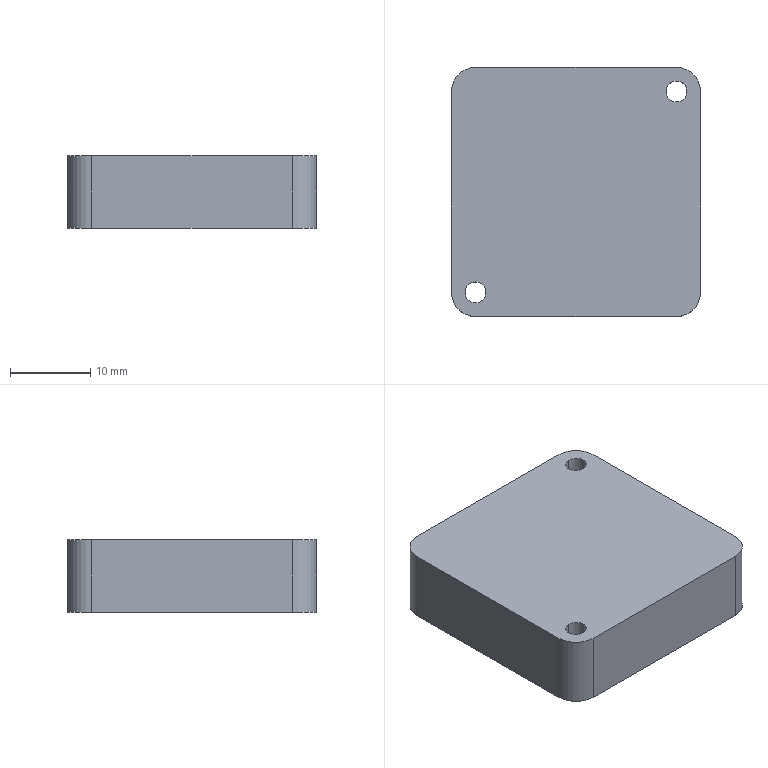NC program | NX | posted with a generic post | part box 31 x 31 x 9 mm
Whole program:
N10 G17 G21 G94 G90
(FLOOR_WALL_COPY , TOOL : D63)
N12 T01 M6
N14 G54
N16 G17 G0 G90 X-50. Y0. S6500 M3
N18 G43 Z30. H1
N20 Z5.
N22 G94 G1 Z2. F1250.
N24 X-47.
N26 X47.
N28 X50.
N30 Z5.
N32 G0 Z30.
N34 X-50.
N36 Z4.
N38 G1 Z1.
N40 X-47.
N42 X47.
N44 X50.
N46 Z4.
N48 G0 Z30.
N50 X-50.
N52 Z3.
N54 G1 Z0.
N56 X-47.
N58 X47.
N60 X50.
N62 Z3.
N64 G0 Z30.
N66 M5
N68 M2